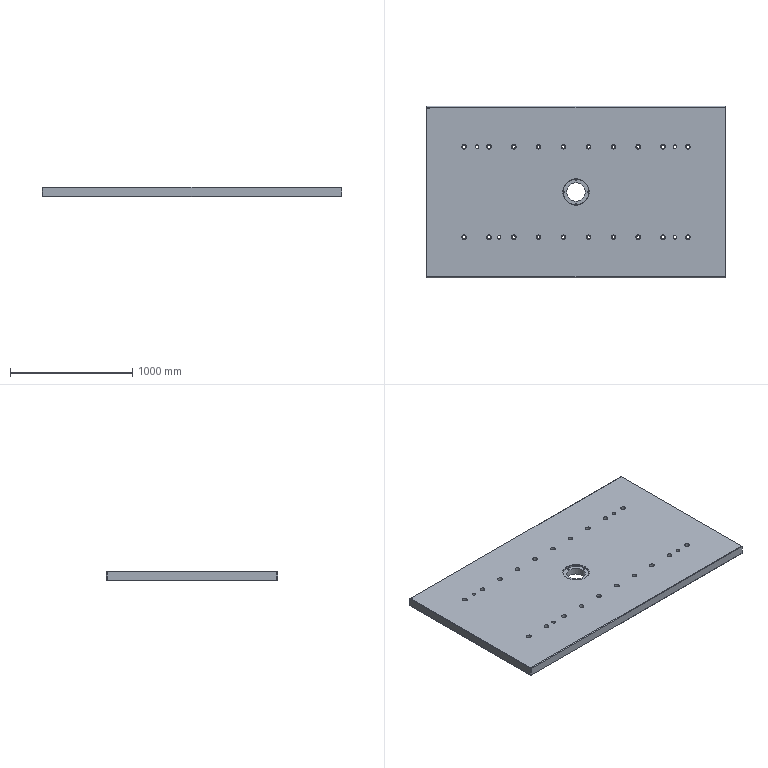Part | STEP file | solid 106 | 1 solid | 120 faces | box 2450 x 1400 x 75.5 mm | volume 255795045 mm3 | plane 58 | cylinder 57 | cone 5 | commonest cylinder face diameters 26 x20 39 x20 5 x6 6.5 x4 30 x4 150 x1